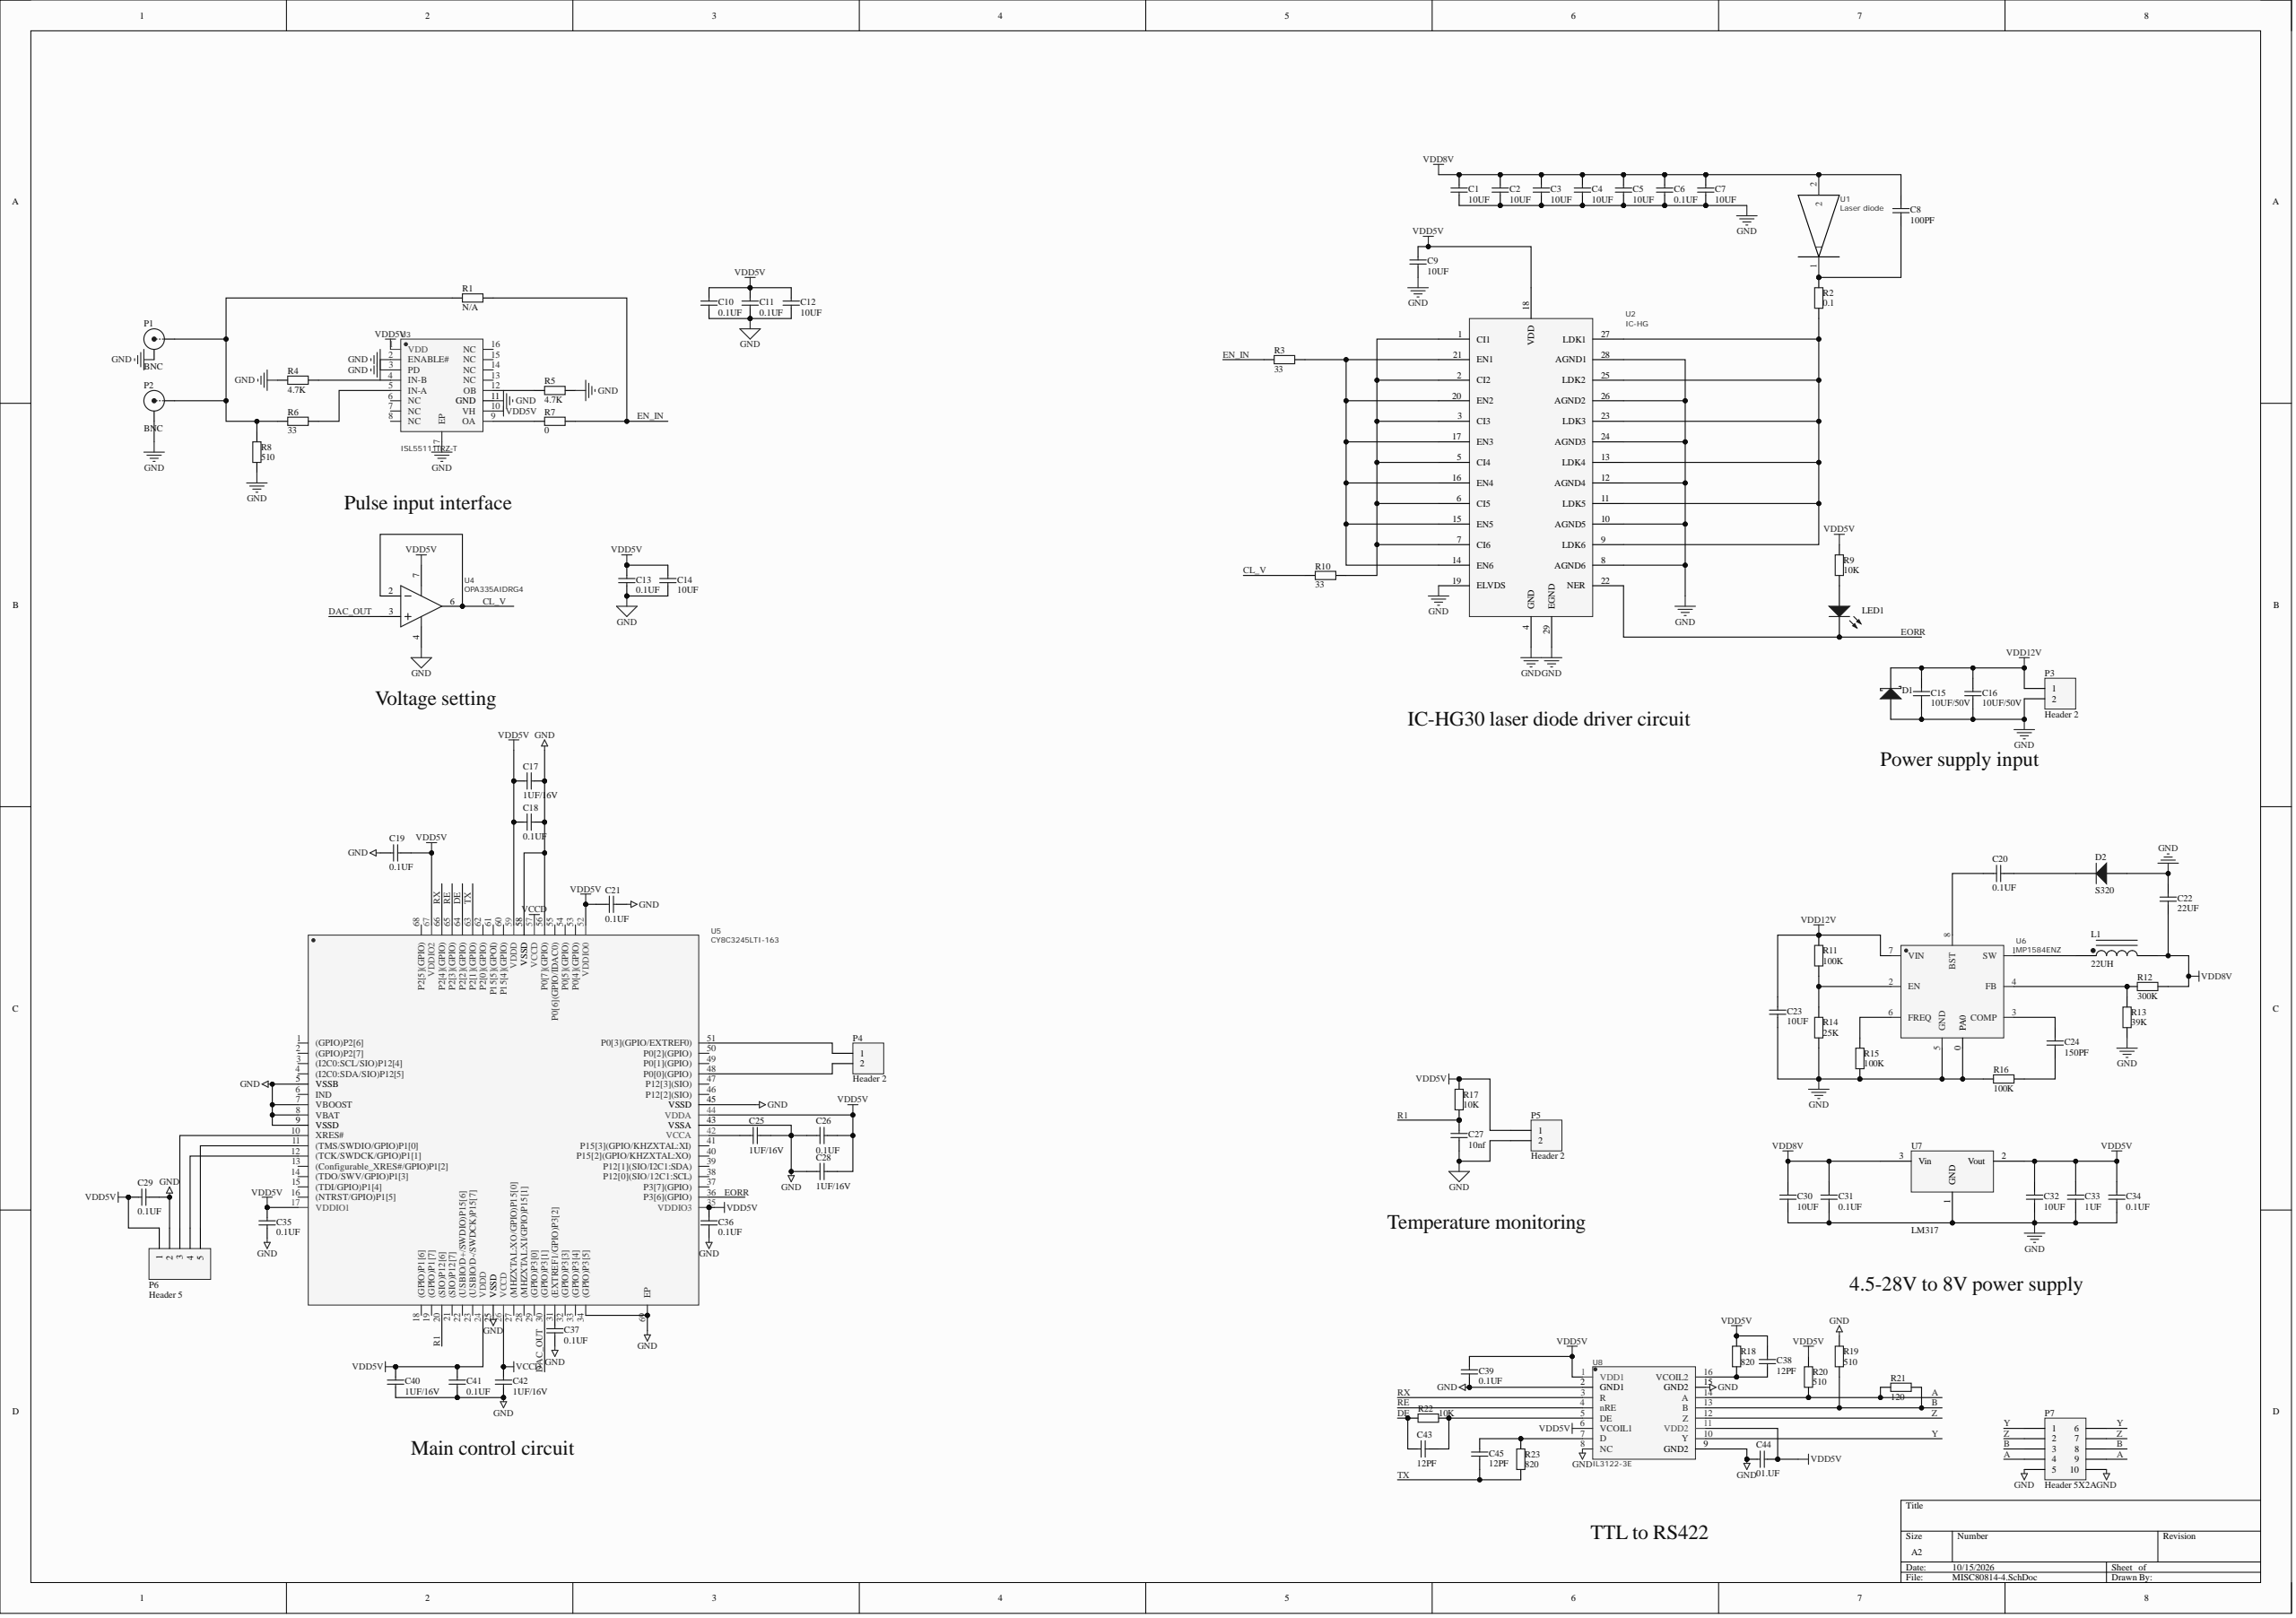Circuit board | Altium Designer | 87 parts | 46 nets
Bill of materials:
Comment,Description,Designator,Footprint,LibRef,Quantity
"10UF","Capacitor (Semiconductor SIM Model)","C1, C2, C3, C4, C5, C7, C9, C12, C14, C23, C30, C32","C0603","Cap Semi","12"
"0.1UF","Capacitor (Semiconductor SIM Model)","C6, C10, C11, C13, C18, C19, C20, C21, C26, C29, C31, C34, C35, C36, C37, C39, C41","C0603","Cap Semi","17"
"100PF","Capacitor (Semiconductor SIM Model)","C8","C0603","Cap Semi","1"
"10UF/50V","Capacitor (Semiconductor SIM Model)","C15, C16","C1206","Cap Semi","2"
"1UF/16V","Capacitor (Semiconductor SIM Model)","C17, C25, C28, C40, C42","C1206","Cap Semi","5"
"22UF","Capacitor (Semiconductor SIM Model)","C22","C0603","Cap Semi","1"
"150PF","Capacitor (Semiconductor SIM Model)","C24","C0603","Cap Semi","1"
"10nf","Capacitor (Semiconductor SIM Model)","C27","C0603","Cap Semi","1"
"1UF","Capacitor (Semiconductor SIM Model)","C33","C0603","Cap Semi","1"
"12PF","Capacitor (Semiconductor SIM Model)","C38, C43, C45","C0603","Cap Semi","3"
"01.UF","Capacitor (Semiconductor SIM Model)","C44","C0603","Cap Semi","1"
"D Schottky","Schottky Diode","D1","SMB","D Schottky","1"
"S320","Default Diode","D2","SMC","Diode","1"
"22UH","Magnetic-Core Inductor with Winding Polarity Marking","L1","DIODE_SMC","Inductor Iron Dot","1"
"LED2","Typical RED, GREEN, YELLOW, AMBER GaAs LED","LED1","3.2X1.6X1.1","LED2","1"
"BNC","BNC Elbow Connector","P1, P2","BNC_RA CON","BNC","2"
"Header 2","Header, 2-Pin","P3, P4, P5","HDR1X2","Header 2","3"
"Header 5","Header, 5-Pin","P6","HDR1X5","Header 5","1"
"Header 5X2A","Header, 5-Pin, Dual row","P7","HDR2X5_CEN","Header 5X2A","1"
"N/A","Resistor","R1","J1-0603","Res2","1"
"0.1","Resistor","R2","J1-0603","Res2","1"
"33","Resistor","R3, R6, R10","J1-0603","Res2","3"
"4.7K","Resistor","R4, R5","J1-0603","Res2","2"
"0","Resistor","R7","J1-0603","Res2","1"
"510","Resistor","R8, R19, R20","J1-0603","Res2","3"
"10K","Resistor","R9, R17, R22","J1-0603","Res2","3"
"100K","Resistor","R11, R15, R16","J1-0603","Res2","3"
"300K","Resistor","R12","J1-0603","Res2","1"
"39K","Resistor","R13","J1-0603","Res2","1"
"25K","Resistor","R14","J1-0603","Res2","1"
"820","Resistor","R18, R23","J1-0603","Res2","2"
"120","Resistor","R21","J1-0603","Res2","1"
"Laser diode","","U1","激光二极管","激光二极管","1"
"IC-HG","","U2","QFN28-5X5","IC-HG","1"
"ISL55111IRZ-T","","U3","QFN-16_L4.0-W4.0-P0.65-BL-EP2.6","ISL55111IRZ-T","1"
"OPA335AIDRG4","","U4","SOP8","OPA335AIDRG4","1"
"CY8C3245LTI-163","","U5","QFN-68_L8.0-W8.0-P0.40-TL-EP5.7","CY8C3245LTI-163","1"
"MP1584ENZ","","U6","MP1548EN","MP1584ENZ_own","1"
"LM317","Adjustable linear regulator IC","U7","TO220A","LM317","1"
"IL3122-3E","","U8","SOIC-16_L9.9-W3.9-P1.27-LS6.0-BL","IL3122-3E","1"
Netlist (Protel format):
[
C1
C0603
10UF



]
[
C2
C0603
10UF



]
[
C3
C0603
10UF



]
[
C4
C0603
10UF



]
[
C5
C0603
10UF



]
[
C6
C0603
0.1UF



]
[
C7
C0603
10UF



]
[
C8
C0603
100PF



]
[
C9
C0603
10UF



]
[
C10
C0603
0.1UF



]
[
C11
C0603
0.1UF



]
[
C12
C0603
10UF



]
[
C13
C0603
0.1UF



]
[
C14
C0603
10UF



]
[
C15
C1206
10UF/50V



]
[
C16
C1206
10UF/50V



]
[
C17
C1206
1UF/16V



]
[
C18
C0603
0.1UF



]
[
C19
C0603
0.1UF



]
[
C20
C0603
0.1UF



]
[
C21
C0603
0.1UF



]
[
C22
C0603
22UF



]
[
C23
C0603
10UF



]
[
C24
C0603
150PF



]
[
C25
C1206
1UF/16V



]
[
C26
C0603
0.1UF



]
[
C27
C0603
10nf



]
[
C28
C1206
1UF/16V



]
[
C29
C0603
0.1UF



]
[
C30
C0603
10UF



]
[
C31
C0603
0.1UF



]
[
C32
C0603
10UF



]
[
C33
C0603
1UF



]
[
C34
C0603
0.1UF



]
[
C35
C0603
0.1UF



]
[
C36
C0603
0.1UF



]
[
C37
C0603
0.1UF



]
[
C38
C0603
12PF



]
[
C39
C0603
0.1UF



]
[
C40
C1206
1UF/16V



]
[
C41
C0603
0.1UF



]
[
C42
C1206
1UF/16V



]
[
C43
C0603
12PF



]
[
C44
C0603
01.UF



]
[
C45
C0603
12PF



]
[
D1
SMB
D Schottky



]
[
D2
SMC
S320



]
[
L1
DIODE_SMC
22UH



]
[
LED1
3.2X1.6X1.1
LED2



]
[
P1
BNC_RA CON
BNC



]
[
P2
BNC_RA CON
BNC



]
[
P3
HDR1X2
Header 2



]
[
P4
HDR1X2
Header 2



]
[
P5
HDR1X2
Header 2



]
[
P6
HDR1X5
Header 5



]
[
P7
HDR2X5_CEN
Header 5X2A



]
[
R1
J1-0603
N/A



]
[
R2
J1-0603
0.1



]
[
R3
J1-0603
33



]
[
R4
J1-0603
4.7K



]
[
R5
J1-0603
4.7K



]
[
R6
J1-0603
33



]
[
R7
J1-0603
0



]
[
R8
J1-0603
510



]
[
R9
J1-0603
10K



]
[
R10
J1-0603
33



]
[
R11
J1-0603
100K



]
[
R12
J1-0603
300K



]
[
R13
J1-0603
39K



]
[
R14
J1-0603
25K



]
[
R15
J1-0603
100K



]
[
R16
J1-0603
100K



]
[
R17
J1-0603
10K



]
[
R18
J1-0603
820



]
[
R19
J1-0603
510



]
[
R20
J1-0603
510



]
[
R21
J1-0603
120



]
[
R22
J1-0603
10K



]
[
R23
J1-0603
820



]
[
U1
激光二极管
Laser diode



]
[
U2
QFN28-5X5
IC-HG



]
[
U3
QFN-16_L4.0-W4.0-P0.65-BL-EP2.6
ISL55111IRZ-T



]
[
U4
SOP8
OPA335AIDRG4



]
[
U5
QFN-68_L8.0-W8.0-P0.40-TL-EP5.7
CY8C3245LTI-163



]
[
U6
MP1548EN
MP1584ENZ



]
[
U7
TO220A
LM317



]
[
U8
SOIC-16_L9.9-W3.9-P1.27-LS6.0-BL
IL3122-3E



]
(
Z
P7-2
P7-7
U8-12
)
(
Y
P7-1
P7-6
U8-10
)
(
VDD12V
C15-2
C16-2
C23-1
D1-2
P3-1
R11-2
U6-7
)
(
VDD8V
C1-2
C2-2
C3-2
C4-2
C5-2
C6-2
C7-2
C8-2
C22-2
C30-1
C31-1
L1-2
R12-1
U1-2
U7-3
)
(
VDD5V
C9-2
C10-2
C11-2
C12-2
C13-2
C14-2
C17-2
C18-2
C19-1
C21-2
C26-1
C28-1
C29-1
C32-1
C33-1
C34-1
C35-2
C36-1
C38-2
C39-1
C40-1
C41-1
C44-1
P5-1
P6-1
R9-2
R17-2
R18-1
R20-1
U2-18
U3-1
U3-10
U4-7
U5-17
U5-24
U5-35
U5-44
U5-52
U5-59
U5-67
U7-2
U8-1
U8-6
U8-11
)
(
VCCD
C42-1
U5-26
U5-57
)
(
TX
C45-1
R23-1
U5-63
)
(
RX
U5-66
U8-3
)
(
RE
U5-65
U8-4
)
(
R1
C27-1
R17-1
U5-20
)
(
NetR15_2
R15-2
U6-6
)
(
NetR12_2
R12-2
R13-1
U6-4
)
(
NetR11_1
R11-1
R14-2
U6-2
)
(
NetR10_1
R10-1
U2-1
U2-2
U2-3
U2-5
U2-6
U2-7
)
(
NetR7_2
R7-2
U3-9
)
(
NetR6_1
R6-1
U3-5
)
(
NetR5_2
R5-2
U3-12
)
(
NetR4_1
R4-1
U3-4
)
(
NetR3_1
R3-1
U2-14
U2-15
U2-16
U2-17
U2-20
U2-21
)
(
NetR2_1
R2-1
U2-9
U2-11
U2-13
U2-23
U2-25
U2-27
)
(
NetP6_5
P6-5
U5-11
)
(
NetP6_4
P6-4
U5-12
)
(
NetP6_3
P6-3
U5-10
)
(
NetP4_2
P4-2
U5-48
)
(
NetP4_1
P4-1
U5-51
)
(
NetP1_1
P1-1
P2-1
R1-2
R6-2
R8-1
)
(
NetLED1_1
LED1-1
R9-1
)
(
NetL1_1
L1-1
U6-1
)
(
NetC45_2
C45-2
R23-2
U8-7
)
(
NetC43_2
C43-2
R22-1
U8-5
)
(
NetC38_1
C38-1
R18-2
U8-16
)
(
NetC37_1
C37-1
U5-31
)
(
NetC25_2
C25-2
U5-42
)
(
NetC24_2
C24-2
R16-2
)
(
NetC24_1
C24-1
U6-3
)
(
NetC20_2
C20-2
U6-8
)
(
NetC20_1
C20-1
D2-2
)
(
NetC8_1
C8-1
R2-2
U1-1
)
(
GND
C1-1
C2-1
C3-1
C4-1
C5-1
C6-1
C7-1
C9-1
C10-1
C11-1
C12-1
C13-1
C14-1
C15-1
C16-1
C17-1
C18-1
C19-2
C21-1
C22-1
C23-2
C25-1
C26-2
C27-2
C28-2
C29-2
C30-2
C31-2
C32-2
C33-2
C34-2
C35-1
C36-2
C37-2
C39-2
C40-2
C41-2
C42-2
C44-2
D1-1
D2-1
P1-2
P2-2
P3-2
P5-2
P6-2
P7-5
P7-10
R4-2
R5-1
R8-2
R13-2
R14-1
R15-1
R16-1
R19-1
U2-4
U2-8
U2-10
U2-12
U2-19
U2-24
U2-26
U2-28
U2-29
U3-2
U3-3
U3-11
U3-17
U4-4
U5-5
U5-7
U5-8
U5-9
U5-25
U5-34
U5-43
U5-45
U5-56
U5-58
U5-69
U6-0
U6-5
U7-1
U8-2
U8-8
U8-9
U8-15
)
(
EORR
LED1-2
U2-22
U5-36
)
(
EN_IN
R1-1
R3-2
R7-1
)
(
DE
C43-1
R22-2
U5-64
)
(
DAC_OUT
U4-3
U5-30
)
(
CL_V
R10-2
U4-2
U4-6
)
(
B
P7-3
P7-8
R19-2
R21-2
U8-13
)
(
A
P7-4
P7-9
R20-2
R21-1
U8-14
)